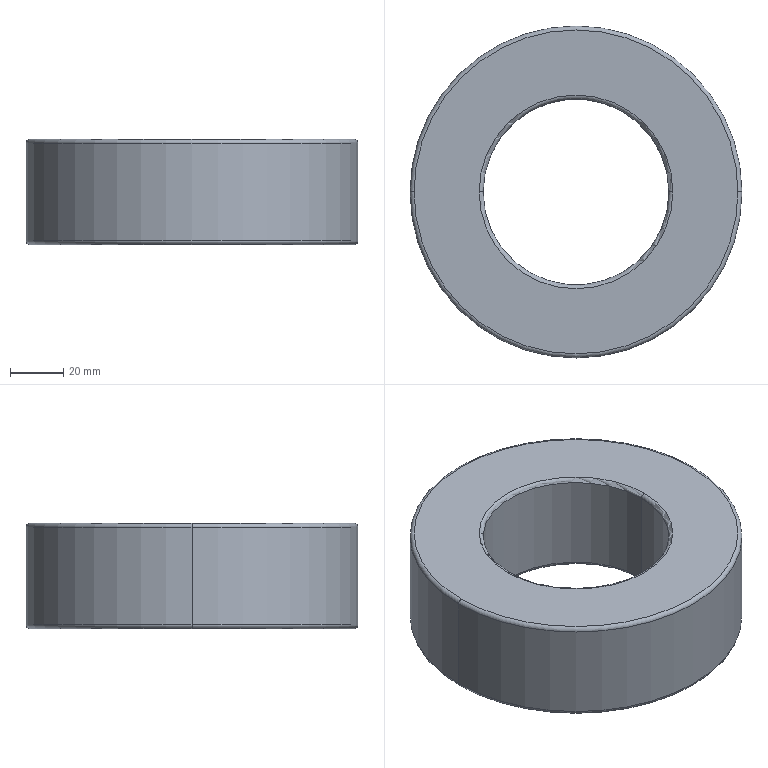Part | SolidWorks | features BaseBody 1 | 1 solid | 14 faces | box 125 x 125 x 39.7 mm | volume 333817 mm3 | torus 8 | cylinder 4 | plane 2 | commonest cylinder face diameters 70 x2 125 x2
STEP:
#1=CARTESIAN_POINT('',(-36.5,0.,-19.85));
#2=VERTEX_POINT('',#1);
#3=CARTESIAN_POINT('',(36.5,0.,-19.85));
#4=VERTEX_POINT('',#3);
#5=CARTESIAN_POINT('',(0.,0.,-19.85));
#6=DIRECTION('',(0.,0.,-1.));
#7=DIRECTION('',(-1.,0.,0.));
#8=AXIS2_PLACEMENT_3D('',#5,#6,#7);
#9=CIRCLE('',#8,36.5);
#10=EDGE_CURVE('',#2,#4,#9,.T.);
#11=ORIENTED_EDGE('',*,*,#10,.T.);
#12=CARTESIAN_POINT('',(35.,0.,-18.35));
#13=VERTEX_POINT('',#12);
#14=CARTESIAN_POINT('',(36.5,0.,-18.35));
#15=DIRECTION('',(0.,1.,0.));
#16=DIRECTION('',(-1.,0.,0.));
#17=AXIS2_PLACEMENT_3D('',#14,#15,#16);
#18=CIRCLE('',#17,1.5);
#19=EDGE_CURVE('',#4,#13,#18,.T.);
#20=ORIENTED_EDGE('',*,*,#19,.T.);
#21=CARTESIAN_POINT('',(-35.,0.,-18.35));
#22=VERTEX_POINT('',#21);
#23=CARTESIAN_POINT('',(0.,0.,-18.35));
#24=DIRECTION('',(0.,0.,-1.));
#25=DIRECTION('',(-1.,0.,0.));
#26=AXIS2_PLACEMENT_3D('',#23,#24,#25);
#27=CIRCLE('',#26,35.);
#28=EDGE_CURVE('',#22,#13,#27,.T.);
#29=ORIENTED_EDGE('',*,*,#28,.F.);
#30=CARTESIAN_POINT('',(-36.5,0.,-18.35));
#31=DIRECTION('',(0.,-1.,0.));
#32=DIRECTION('',(0.,0.,-1.));
#33=AXIS2_PLACEMENT_3D('',#30,#31,#32);
#34=CIRCLE('',#33,1.5);
#35=EDGE_CURVE('',#2,#22,#34,.T.);
#36=ORIENTED_EDGE('',*,*,#35,.F.);
#37=EDGE_LOOP('',(#11,#20,#29,#36));
#38=FACE_OUTER_BOUND('',#37,.T.);
#39=CARTESIAN_POINT('',(0.,0.,-18.35));
#40=DIRECTION('',(0.,0.,-1.));
#41=DIRECTION('',(-1.,0.,0.));
#42=AXIS2_PLACEMENT_3D('',#39,#40,#41);
#43=TOROIDAL_SURFACE('',#42,36.5,1.5);
#44=ADVANCED_FACE('',(#38),#43,.T.);
#45=CARTESIAN_POINT('',(35.,0.,18.35));
#46=VERTEX_POINT('',#45);
#47=CARTESIAN_POINT('',(-35.,0.,18.35));
#48=VERTEX_POINT('',#47);
#49=CARTESIAN_POINT('',(0.,0.,18.35));
#50=DIRECTION('',(0.,0.,-1.));
#51=DIRECTION('',(-1.,0.,0.));
#52=AXIS2_PLACEMENT_3D('',#49,#50,#51);
#53=CIRCLE('',#52,35.);
#54=EDGE_CURVE('',#46,#48,#53,.T.);
#55=ORIENTED_EDGE('',*,*,#54,.F.);
#56=CARTESIAN_POINT('',(35.,0.,-50.));
#57=DIRECTION('',(0.,0.,-1.));
#58=VECTOR('',#57,1000.);
#59=LINE('',#56,#58);
#60=EDGE_CURVE('',#46,#13,#59,.T.);
#61=ORIENTED_EDGE('',*,*,#60,.T.);
#62=CARTESIAN_POINT('',(0.,0.,-18.35));
#63=DIRECTION('',(0.,0.,-1.));
#64=DIRECTION('',(-1.,0.,0.));
#65=AXIS2_PLACEMENT_3D('',#62,#63,#64);
#66=CIRCLE('',#65,35.);
#67=EDGE_CURVE('',#13,#22,#66,.T.);
#68=ORIENTED_EDGE('',*,*,#67,.T.);
#69=CARTESIAN_POINT('',(-35.,0.,-50.));
#70=DIRECTION('',(0.,0.,-1.));
#71=VECTOR('',#70,1000.);
#72=LINE('',#69,#71);
#73=EDGE_CURVE('',#48,#22,#72,.T.);
#74=ORIENTED_EDGE('',*,*,#73,.F.);
#75=EDGE_LOOP('',(#55,#61,#68,#74));
#76=FACE_OUTER_BOUND('',#75,.T.);
#77=CARTESIAN_POINT('',(0.,0.,-50.));
#78=DIRECTION('',(0.,0.,-1.));
#79=DIRECTION('',(-1.,0.,0.));
#80=AXIS2_PLACEMENT_3D('',#77,#78,#79);
#81=CYLINDRICAL_SURFACE('',#80,35.);
#82=ADVANCED_FACE('',(#76),#81,.F.);
#83=CARTESIAN_POINT('',(-62.5,0.,-18.35));
#84=VERTEX_POINT('',#83);
#85=CARTESIAN_POINT('',(62.5,0.,-18.35));
#86=VERTEX_POINT('',#85);
#87=CARTESIAN_POINT('',(0.,0.,-18.35));
#88=DIRECTION('',(0.,0.,-1.));
#89=DIRECTION('',(-1.,0.,0.));
#90=AXIS2_PLACEMENT_3D('',#87,#88,#89);
#91=CIRCLE('',#90,62.5);
#92=EDGE_CURVE('',#84,#86,#91,.T.);
#93=ORIENTED_EDGE('',*,*,#92,.T.);
#94=CARTESIAN_POINT('',(61.,0.,-19.85));
#95=VERTEX_POINT('',#94);
#96=CARTESIAN_POINT('',(61.,0.,-18.35));
#97=DIRECTION('',(0.,1.,0.));
#98=DIRECTION('',(-1.,0.,0.));
#99=AXIS2_PLACEMENT_3D('',#96,#97,#98);
#100=CIRCLE('',#99,1.5);
#101=EDGE_CURVE('',#86,#95,#100,.T.);
#102=ORIENTED_EDGE('',*,*,#101,.T.);
#103=CARTESIAN_POINT('',(-61.,0.,-19.85));
#104=VERTEX_POINT('',#103);
#105=CARTESIAN_POINT('',(0.,0.,-19.85));
#106=DIRECTION('',(0.,0.,-1.));
#107=DIRECTION('',(-1.,0.,0.));
#108=AXIS2_PLACEMENT_3D('',#105,#106,#107);
#109=CIRCLE('',#108,61.);
#110=EDGE_CURVE('',#104,#95,#109,.T.);
#111=ORIENTED_EDGE('',*,*,#110,.F.);
#112=CARTESIAN_POINT('',(-61.,0.,-18.35));
#113=DIRECTION('',(0.,-1.,0.));
#114=DIRECTION('',(0.,0.,-1.));
#115=AXIS2_PLACEMENT_3D('',#112,#113,#114);
#116=CIRCLE('',#115,1.5);
#117=EDGE_CURVE('',#84,#104,#116,.T.);
#118=ORIENTED_EDGE('',*,*,#117,.F.);
#119=EDGE_LOOP('',(#93,#102,#111,#118));
#120=FACE_OUTER_BOUND('',#119,.T.);
#121=CARTESIAN_POINT('',(0.,0.,-18.35));
#122=DIRECTION('',(0.,0.,-1.));
#123=DIRECTION('',(-1.,0.,0.));
#124=AXIS2_PLACEMENT_3D('',#121,#122,#123);
#125=TOROIDAL_SURFACE('',#124,61.,1.5);
#126=ADVANCED_FACE('',(#120),#125,.T.);
#127=CARTESIAN_POINT('',(0.,0.,18.35));
#128=DIRECTION('',(0.,0.,-1.));
#129=DIRECTION('',(-1.,0.,0.));
#130=AXIS2_PLACEMENT_3D('',#127,#128,#129);
#131=CIRCLE('',#130,35.);
#132=EDGE_CURVE('',#48,#46,#131,.T.);
#133=ORIENTED_EDGE('',*,*,#132,.T.);
#134=CARTESIAN_POINT('',(36.5,0.,19.85));
#135=VERTEX_POINT('',#134);
#136=CARTESIAN_POINT('',(36.5,0.,18.35));
#137=DIRECTION('',(0.,1.,0.));
#138=DIRECTION('',(-1.,0.,0.));
#139=AXIS2_PLACEMENT_3D('',#136,#137,#138);
#140=CIRCLE('',#139,1.5);
#141=EDGE_CURVE('',#46,#135,#140,.T.);
#142=ORIENTED_EDGE('',*,*,#141,.T.);
#143=CARTESIAN_POINT('',(-36.5,0.,19.85));
#144=VERTEX_POINT('',#143);
#145=CARTESIAN_POINT('',(0.,0.,19.85));
#146=DIRECTION('',(0.,0.,-1.));
#147=DIRECTION('',(-1.,0.,0.));
#148=AXIS2_PLACEMENT_3D('',#145,#146,#147);
#149=CIRCLE('',#148,36.5);
#150=EDGE_CURVE('',#144,#135,#149,.T.);
#151=ORIENTED_EDGE('',*,*,#150,.F.);
#152=CARTESIAN_POINT('',(-36.5,0.,18.35));
#153=DIRECTION('',(0.,-1.,0.));
#154=DIRECTION('',(0.,0.,-1.));
#155=AXIS2_PLACEMENT_3D('',#152,#153,#154);
#156=CIRCLE('',#155,1.5);
#157=EDGE_CURVE('',#48,#144,#156,.T.);
#158=ORIENTED_EDGE('',*,*,#157,.F.);
#159=EDGE_LOOP('',(#133,#142,#151,#158));
#160=FACE_OUTER_BOUND('',#159,.T.);
#161=CARTESIAN_POINT('',(0.,0.,18.35));
#162=DIRECTION('',(0.,0.,-1.));
#163=DIRECTION('',(-1.,0.,0.));
#164=AXIS2_PLACEMENT_3D('',#161,#162,#163);
#165=TOROIDAL_SURFACE('',#164,36.5,1.5);
#166=ADVANCED_FACE('',(#160),#165,.T.);
#167=CARTESIAN_POINT('',(-62.5,0.,18.35));
#168=VERTEX_POINT('',#167);
#169=CARTESIAN_POINT('',(62.5,0.,18.35));
#170=VERTEX_POINT('',#169);
#171=CARTESIAN_POINT('',(0.,0.,18.35));
#172=DIRECTION('',(0.,0.,-1.));
#173=DIRECTION('',(-1.,0.,0.));
#174=AXIS2_PLACEMENT_3D('',#171,#172,#173);
#175=CIRCLE('',#174,62.5);
#176=EDGE_CURVE('',#168,#170,#175,.T.);
#177=ORIENTED_EDGE('',*,*,#176,.T.);
#178=CARTESIAN_POINT('',(62.5,0.,-50.));
#179=DIRECTION('',(0.,0.,-1.));
#180=VECTOR('',#179,1000.);
#181=LINE('',#178,#180);
#182=EDGE_CURVE('',#170,#86,#181,.T.);
#183=ORIENTED_EDGE('',*,*,#182,.T.);
#184=ORIENTED_EDGE('',*,*,#92,.F.);
#185=CARTESIAN_POINT('',(-62.5,0.,-50.));
#186=DIRECTION('',(0.,0.,-1.));
#187=VECTOR('',#186,1000.);
#188=LINE('',#185,#187);
#189=EDGE_CURVE('',#168,#84,#188,.T.);
#190=ORIENTED_EDGE('',*,*,#189,.F.);
#191=EDGE_LOOP('',(#177,#183,#184,#190));
#192=FACE_OUTER_BOUND('',#191,.T.);
#193=CARTESIAN_POINT('',(0.,0.,-50.));
#194=DIRECTION('',(0.,0.,-1.));
#195=DIRECTION('',(-1.,0.,0.));
#196=AXIS2_PLACEMENT_3D('',#193,#194,#195);
#197=CYLINDRICAL_SURFACE('',#196,62.5);
#198=ADVANCED_FACE('',(#192),#197,.T.);
#199=CARTESIAN_POINT('',(-61.,0.,19.85));
#200=VERTEX_POINT('',#199);
#201=CARTESIAN_POINT('',(61.,0.,19.85));
#202=VERTEX_POINT('',#201);
#203=CARTESIAN_POINT('',(0.,0.,19.85));
#204=DIRECTION('',(0.,0.,-1.));
#205=DIRECTION('',(-1.,0.,0.));
#206=AXIS2_PLACEMENT_3D('',#203,#204,#205);
#207=CIRCLE('',#206,61.);
#208=EDGE_CURVE('',#200,#202,#207,.T.);
#209=ORIENTED_EDGE('',*,*,#208,.T.);
#210=CARTESIAN_POINT('',(61.,0.,18.35));
#211=DIRECTION('',(0.,1.,0.));
#212=DIRECTION('',(-1.,0.,0.));
#213=AXIS2_PLACEMENT_3D('',#210,#211,#212);
#214=CIRCLE('',#213,1.5);
#215=EDGE_CURVE('',#202,#170,#214,.T.);
#216=ORIENTED_EDGE('',*,*,#215,.T.);
#217=ORIENTED_EDGE('',*,*,#176,.F.);
#218=CARTESIAN_POINT('',(-61.,0.,18.35));
#219=DIRECTION('',(0.,-1.,0.));
#220=DIRECTION('',(0.,0.,-1.));
#221=AXIS2_PLACEMENT_3D('',#218,#219,#220);
#222=CIRCLE('',#221,1.5);
#223=EDGE_CURVE('',#200,#168,#222,.T.);
#224=ORIENTED_EDGE('',*,*,#223,.F.);
#225=EDGE_LOOP('',(#209,#216,#217,#224));
#226=FACE_OUTER_BOUND('',#225,.T.);
#227=CARTESIAN_POINT('',(0.,0.,18.35));
#228=DIRECTION('',(0.,0.,-1.));
#229=DIRECTION('',(-1.,0.,0.));
#230=AXIS2_PLACEMENT_3D('',#227,#228,#229);
#231=TOROIDAL_SURFACE('',#230,61.,1.5);
#232=ADVANCED_FACE('',(#226),#231,.T.);
#233=ORIENTED_EDGE('',*,*,#215,.F.);
#234=CARTESIAN_POINT('',(0.,0.,19.85));
#235=DIRECTION('',(0.,0.,-1.));
#236=DIRECTION('',(-1.,0.,0.));
#237=AXIS2_PLACEMENT_3D('',#234,#235,#236);
#238=CIRCLE('',#237,61.);
#239=EDGE_CURVE('',#202,#200,#238,.T.);
#240=ORIENTED_EDGE('',*,*,#239,.T.);
#241=ORIENTED_EDGE('',*,*,#223,.T.);
#242=CARTESIAN_POINT('',(0.,0.,18.35));
#243=DIRECTION('',(0.,0.,-1.));
#244=DIRECTION('',(-1.,0.,0.));
#245=AXIS2_PLACEMENT_3D('',#242,#243,#244);
#246=CIRCLE('',#245,62.5);
#247=EDGE_CURVE('',#170,#168,#246,.T.);
#248=ORIENTED_EDGE('',*,*,#247,.F.);
#249=EDGE_LOOP('',(#233,#240,#241,#248));
#250=FACE_OUTER_BOUND('',#249,.T.);
#251=CARTESIAN_POINT('',(0.,0.,18.35));
#252=DIRECTION('',(0.,0.,-1.));
#253=DIRECTION('',(-1.,0.,0.));
#254=AXIS2_PLACEMENT_3D('',#251,#252,#253);
#255=TOROIDAL_SURFACE('',#254,61.,1.5);
#256=ADVANCED_FACE('',(#250),#255,.T.);
#257=ORIENTED_EDGE('',*,*,#150,.T.);
#258=CARTESIAN_POINT('',(0.,0.,19.85));
#259=DIRECTION('',(0.,0.,-1.));
#260=DIRECTION('',(-1.,0.,0.));
#261=AXIS2_PLACEMENT_3D('',#258,#259,#260);
#262=CIRCLE('',#261,36.5);
#263=EDGE_CURVE('',#135,#144,#262,.T.);
#264=ORIENTED_EDGE('',*,*,#263,.T.);
#265=EDGE_LOOP('',(#257,#264));
#266=FACE_BOUND('',#265,.T.);
#267=ORIENTED_EDGE('',*,*,#208,.F.);
#268=ORIENTED_EDGE('',*,*,#239,.F.);
#269=EDGE_LOOP('',(#267,#268));
#270=FACE_OUTER_BOUND('',#269,.T.);
#271=CARTESIAN_POINT('',(0.,61.,19.85));
#272=DIRECTION('',(0.,0.,1.));
#273=DIRECTION('',(1.,0.,0.));
#274=AXIS2_PLACEMENT_3D('',#271,#272,#273);
#275=PLANE('',#274);
#276=ADVANCED_FACE('',(#266,#270),#275,.T.);
#277=ORIENTED_EDGE('',*,*,#182,.F.);
#278=ORIENTED_EDGE('',*,*,#247,.T.);
#279=ORIENTED_EDGE('',*,*,#189,.T.);
#280=CARTESIAN_POINT('',(0.,0.,-18.35));
#281=DIRECTION('',(0.,0.,-1.));
#282=DIRECTION('',(-1.,0.,0.));
#283=AXIS2_PLACEMENT_3D('',#280,#281,#282);
#284=CIRCLE('',#283,62.5);
#285=EDGE_CURVE('',#86,#84,#284,.T.);
#286=ORIENTED_EDGE('',*,*,#285,.F.);
#287=EDGE_LOOP('',(#277,#278,#279,#286));
#288=FACE_OUTER_BOUND('',#287,.T.);
#289=CARTESIAN_POINT('',(0.,0.,-50.));
#290=DIRECTION('',(0.,0.,-1.));
#291=DIRECTION('',(-1.,0.,0.));
#292=AXIS2_PLACEMENT_3D('',#289,#290,#291);
#293=CYLINDRICAL_SURFACE('',#292,62.5);
#294=ADVANCED_FACE('',(#288),#293,.T.);
#295=ORIENTED_EDGE('',*,*,#141,.F.);
#296=ORIENTED_EDGE('',*,*,#54,.T.);
#297=ORIENTED_EDGE('',*,*,#157,.T.);
#298=ORIENTED_EDGE('',*,*,#263,.F.);
#299=EDGE_LOOP('',(#295,#296,#297,#298));
#300=FACE_OUTER_BOUND('',#299,.T.);
#301=CARTESIAN_POINT('',(0.,0.,18.35));
#302=DIRECTION('',(0.,0.,-1.));
#303=DIRECTION('',(-1.,0.,0.));
#304=AXIS2_PLACEMENT_3D('',#301,#302,#303);
#305=TOROIDAL_SURFACE('',#304,36.5,1.5);
#306=ADVANCED_FACE('',(#300),#305,.T.);
#307=ORIENTED_EDGE('',*,*,#101,.F.);
#308=ORIENTED_EDGE('',*,*,#285,.T.);
#309=ORIENTED_EDGE('',*,*,#117,.T.);
#310=CARTESIAN_POINT('',(0.,0.,-19.85));
#311=DIRECTION('',(0.,0.,-1.));
#312=DIRECTION('',(-1.,0.,0.));
#313=AXIS2_PLACEMENT_3D('',#310,#311,#312);
#314=CIRCLE('',#313,61.);
#315=EDGE_CURVE('',#95,#104,#314,.T.);
#316=ORIENTED_EDGE('',*,*,#315,.F.);
#317=EDGE_LOOP('',(#307,#308,#309,#316));
#318=FACE_OUTER_BOUND('',#317,.T.);
#319=CARTESIAN_POINT('',(0.,0.,-18.35));
#320=DIRECTION('',(0.,0.,-1.));
#321=DIRECTION('',(-1.,0.,0.));
#322=AXIS2_PLACEMENT_3D('',#319,#320,#321);
#323=TOROIDAL_SURFACE('',#322,61.,1.5);
#324=ADVANCED_FACE('',(#318),#323,.T.);
#325=ORIENTED_EDGE('',*,*,#60,.F.);
#326=ORIENTED_EDGE('',*,*,#132,.F.);
#327=ORIENTED_EDGE('',*,*,#73,.T.);
#328=ORIENTED_EDGE('',*,*,#28,.T.);
#329=EDGE_LOOP('',(#325,#326,#327,#328));
#330=FACE_OUTER_BOUND('',#329,.T.);
#331=CARTESIAN_POINT('',(0.,0.,-50.));
#332=DIRECTION('',(0.,0.,-1.));
#333=DIRECTION('',(-1.,0.,0.));
#334=AXIS2_PLACEMENT_3D('',#331,#332,#333);
#335=CYLINDRICAL_SURFACE('',#334,35.);
#336=ADVANCED_FACE('',(#330),#335,.F.);
#337=ORIENTED_EDGE('',*,*,#110,.T.);
#338=ORIENTED_EDGE('',*,*,#315,.T.);
#339=EDGE_LOOP('',(#337,#338));
#340=FACE_OUTER_BOUND('',#339,.T.);
#341=ORIENTED_EDGE('',*,*,#10,.F.);
#342=CARTESIAN_POINT('',(0.,0.,-19.85));
#343=DIRECTION('',(0.,0.,-1.));
#344=DIRECTION('',(-1.,0.,0.));
#345=AXIS2_PLACEMENT_3D('',#342,#343,#344);
#346=CIRCLE('',#345,36.5);
#347=EDGE_CURVE('',#4,#2,#346,.T.);
#348=ORIENTED_EDGE('',*,*,#347,.F.);
#349=EDGE_LOOP('',(#341,#348));
#350=FACE_BOUND('',#349,.T.);
#351=CARTESIAN_POINT('',(0.,36.5,-19.85));
#352=DIRECTION('',(0.,0.,-1.));
#353=DIRECTION('',(-1.,0.,0.));
#354=AXIS2_PLACEMENT_3D('',#351,#352,#353);
#355=PLANE('',#354);
#356=ADVANCED_FACE('',(#340,#350),#355,.T.);
#357=ORIENTED_EDGE('',*,*,#19,.F.);
#358=ORIENTED_EDGE('',*,*,#347,.T.);
#359=ORIENTED_EDGE('',*,*,#35,.T.);
#360=ORIENTED_EDGE('',*,*,#67,.F.);
#361=EDGE_LOOP('',(#357,#358,#359,#360));
#362=FACE_OUTER_BOUND('',#361,.T.);
#363=CARTESIAN_POINT('',(0.,0.,-18.35));
#364=DIRECTION('',(0.,0.,-1.));
#365=DIRECTION('',(-1.,0.,0.));
#366=AXIS2_PLACEMENT_3D('',#363,#364,#365);
#367=TOROIDAL_SURFACE('',#366,36.5,1.5);
#368=ADVANCED_FACE('',(#362),#367,.T.);
#369=CLOSED_SHELL('',(#44,#82,#126,#166,#198,#232,#256,#276,#294,#306,#324,#336,#356,#368));
#370=MANIFOLD_SOLID_BREP('',#369);
#371=CARTESIAN_POINT('',(0.,0.,0.));
#372=DIRECTION('',(0.,0.,1.));
#373=DIRECTION('',(1.,0.,0.));
#374=AXIS2_PLACEMENT_3D('',#371,#372,#373);
#375=(LENGTH_UNIT()NAMED_UNIT(*)SI_UNIT(.MILLI.,.METRE.));
#376=UNCERTAINTY_MEASURE_WITH_UNIT(LENGTH_MEASURE(0.00001),#375,'','');
#377=(NAMED_UNIT(*)PLANE_ANGLE_UNIT()SI_UNIT($,.RADIAN.));
#378=(NAMED_UNIT(*)SI_UNIT($,.STERADIAN.)SOLID_ANGLE_UNIT());
#379=(GEOMETRIC_REPRESENTATION_CONTEXT(3)GLOBAL_UNCERTAINTY_ASSIGNED_CONTEXT((#376))GLOBAL_UNIT_ASSIGNED_CONTEXT((#375,#377,#378))REPRESENTATION_CONTEXT('',''));
#380=ADVANCED_BREP_SHAPE_REPRESENTATION('',(#370,#374),#379);